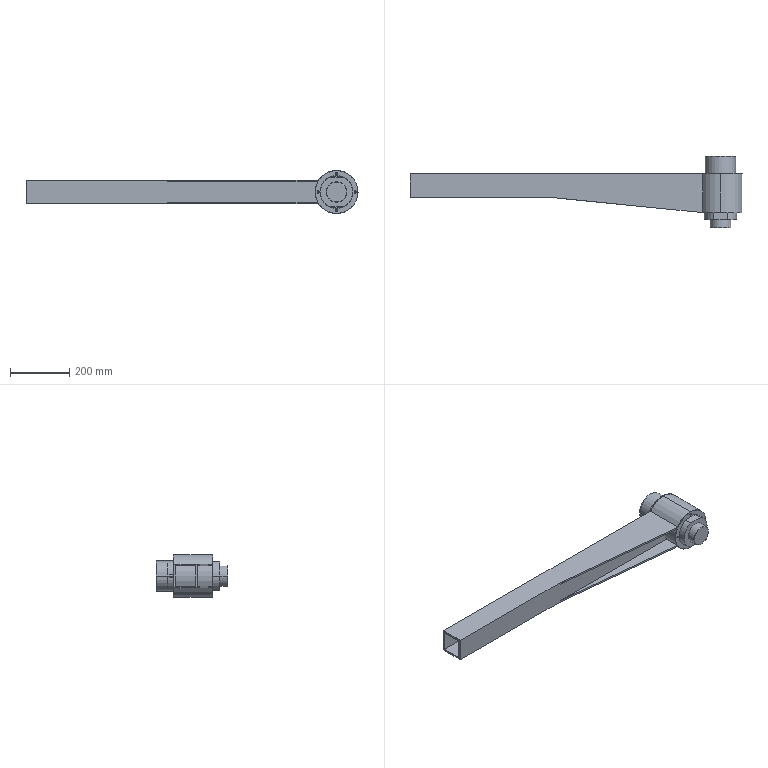Part | SolidWorks | features CompositeCurve 16 | 7 solids | 632 faces | box 1123 x 243 x 145 mm | volume 4299849 mm3 | torus 240 | plane 162 | cone 148 | cylinder 82 | commonest cylinder face diameters 5 x16 7 x16 110 x11 70 x10 145 x9 100 x6